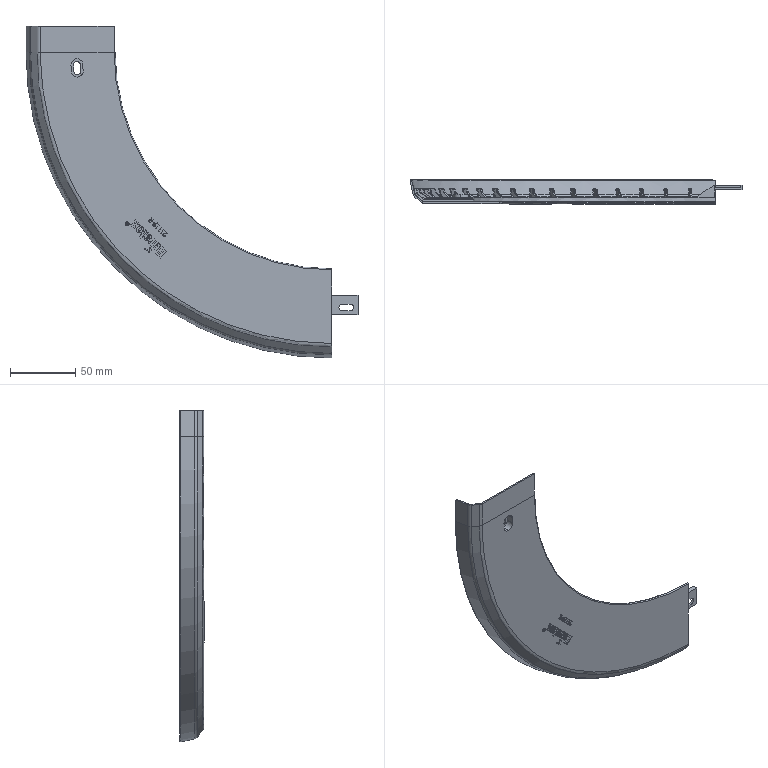Part | STEP file | V00-000000453 | 2 solids | 1753 faces | box 254.244 x 18.951 x 254.244 mm | volume 49463 mm3 | cylinder 554 | torus 394 | plane 370 | spline 219 | sphere 190 | cone 26 | commonest cylinder face diameters 1 x397 2 x40 1.048 x20 375 x19 420 x19 423 x19